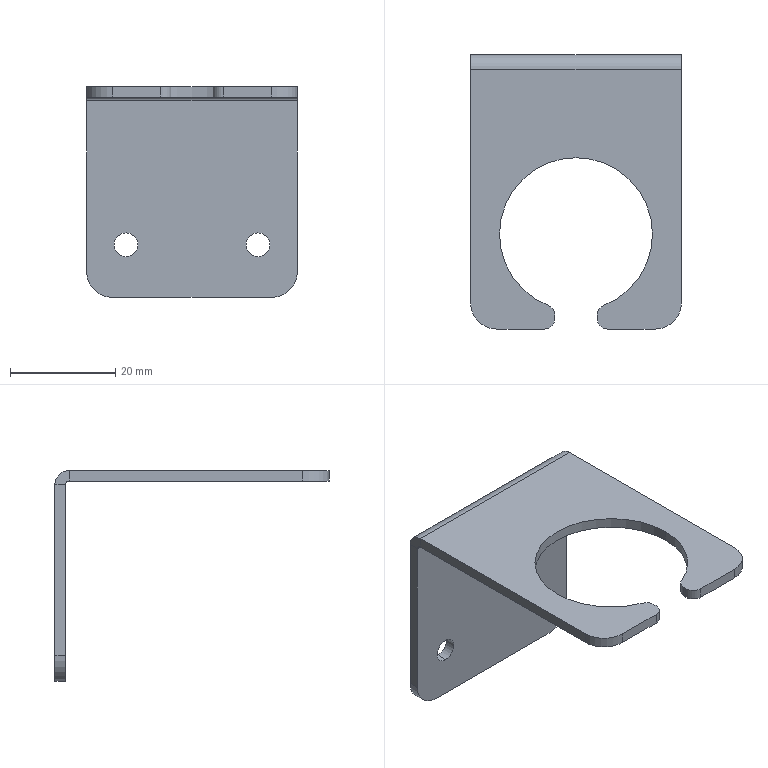Part | STEP file | 02-10 corrugated tube mounting plate (Default) | 1 solid | 32 faces | box 40 x 52 x 40 mm | volume 5649 mm3 | cylinder 17 | plane 15 | commonest cylinder face diameters 4 x4 4.5 x4 10 x4 29 x3 1.473 x1 5.473 x1
STEP:
#1=CARTESIAN_POINT('',(12.5,27.,-32.25));
#2=VERTEX_POINT('',#1);
#3=CARTESIAN_POINT('',(12.5,27.,-27.75));
#4=VERTEX_POINT('',#3);
#5=CARTESIAN_POINT('',(12.5,27.,-30.));
#6=DIRECTION('',(0.,1.,0.));
#7=DIRECTION('',(0.,0.,1.));
#8=AXIS2_PLACEMENT_3D('',#5,#6,#7);
#9=CIRCLE('',#8,2.25);
#10=EDGE_CURVE('',#2,#4,#9,.T.);
#11=ORIENTED_EDGE('',*,*,#10,.T.);
#12=CARTESIAN_POINT('',(12.5,25.,-27.75));
#13=VERTEX_POINT('',#12);
#14=CARTESIAN_POINT('',(12.5,35.,-27.75));
#15=DIRECTION('',(0.,-1.,0.));
#16=VECTOR('',#15,1000.);
#17=LINE('',#14,#16);
#18=EDGE_CURVE('',#4,#13,#17,.T.);
#19=ORIENTED_EDGE('',*,*,#18,.T.);
#20=CARTESIAN_POINT('',(12.5,25.,-32.25));
#21=VERTEX_POINT('',#20);
#22=CARTESIAN_POINT('',(12.5,25.,-30.));
#23=DIRECTION('',(0.,-1.,0.));
#24=DIRECTION('',(0.,0.,1.));
#25=AXIS2_PLACEMENT_3D('',#22,#23,#24);
#26=CIRCLE('',#25,2.25);
#27=EDGE_CURVE('',#13,#21,#26,.T.);
#28=ORIENTED_EDGE('',*,*,#27,.T.);
#29=CARTESIAN_POINT('',(12.5,35.,-32.25));
#30=DIRECTION('',(0.,-1.,0.));
#31=VECTOR('',#30,1000.);
#32=LINE('',#29,#31);
#33=EDGE_CURVE('',#2,#21,#32,.T.);
#34=ORIENTED_EDGE('',*,*,#33,.F.);
#35=EDGE_LOOP('',(#11,#19,#28,#34));
#36=FACE_OUTER_BOUND('',#35,.T.);
#37=CARTESIAN_POINT('',(12.5,35.,-30.));
#38=DIRECTION('',(0.,-1.,0.));
#39=DIRECTION('',(0.,0.,-1.));
#40=AXIS2_PLACEMENT_3D('',#37,#38,#39);
#41=CYLINDRICAL_SURFACE('',#40,2.25);
#42=ADVANCED_FACE('',(#36),#41,.F.);
#43=CARTESIAN_POINT('',(-12.5,27.,-32.25));
#44=VERTEX_POINT('',#43);
#45=CARTESIAN_POINT('',(-12.5,27.,-27.75));
#46=VERTEX_POINT('',#45);
#47=CARTESIAN_POINT('',(-12.5,27.,-30.));
#48=DIRECTION('',(0.,1.,0.));
#49=DIRECTION('',(0.,0.,1.));
#50=AXIS2_PLACEMENT_3D('',#47,#48,#49);
#51=CIRCLE('',#50,2.25);
#52=EDGE_CURVE('',#44,#46,#51,.T.);
#53=ORIENTED_EDGE('',*,*,#52,.T.);
#54=CARTESIAN_POINT('',(-12.5,25.,-27.75));
#55=VERTEX_POINT('',#54);
#56=CARTESIAN_POINT('',(-12.5,35.,-27.75));
#57=DIRECTION('',(0.,-1.,0.));
#58=VECTOR('',#57,1000.);
#59=LINE('',#56,#58);
#60=EDGE_CURVE('',#46,#55,#59,.T.);
#61=ORIENTED_EDGE('',*,*,#60,.T.);
#62=CARTESIAN_POINT('',(-12.5,25.,-32.25));
#63=VERTEX_POINT('',#62);
#64=CARTESIAN_POINT('',(-12.5,25.,-30.));
#65=DIRECTION('',(0.,-1.,0.));
#66=DIRECTION('',(0.,0.,-1.));
#67=AXIS2_PLACEMENT_3D('',#64,#65,#66);
#68=CIRCLE('',#67,2.25);
#69=EDGE_CURVE('',#55,#63,#68,.T.);
#70=ORIENTED_EDGE('',*,*,#69,.T.);
#71=CARTESIAN_POINT('',(-12.5,35.,-32.25));
#72=DIRECTION('',(0.,-1.,0.));
#73=VECTOR('',#72,1000.);
#74=LINE('',#71,#73);
#75=EDGE_CURVE('',#44,#63,#74,.T.);
#76=ORIENTED_EDGE('',*,*,#75,.F.);
#77=EDGE_LOOP('',(#53,#61,#70,#76));
#78=FACE_OUTER_BOUND('',#77,.T.);
#79=CARTESIAN_POINT('',(-12.5,35.,-30.));
#80=DIRECTION('',(0.,-1.,0.));
#81=DIRECTION('',(0.,0.,-1.));
#82=AXIS2_PLACEMENT_3D('',#79,#80,#81);
#83=CYLINDRICAL_SURFACE('',#82,2.25);
#84=ADVANCED_FACE('',(#78),#83,.F.);
#85=CARTESIAN_POINT('',(-14.5,-7.,-2.));
#86=VERTEX_POINT('',#85);
#87=CARTESIAN_POINT('',(-5.273,-20.507,-2.));
#88=VERTEX_POINT('',#87);
#89=CARTESIAN_POINT('',(0.,-7.,-2.));
#90=DIRECTION('',(0.,0.,1.));
#91=DIRECTION('',(1.,0.,0.));
#92=AXIS2_PLACEMENT_3D('',#89,#90,#91);
#93=CIRCLE('',#92,14.5);
#94=EDGE_CURVE('',#86,#88,#93,.T.);
#95=ORIENTED_EDGE('',*,*,#94,.F.);
#96=CARTESIAN_POINT('',(-14.5,-7.,0.));
#97=VERTEX_POINT('',#96);
#98=CARTESIAN_POINT('',(-14.5,-7.,-10.));
#99=DIRECTION('',(0.,0.,1.));
#100=VECTOR('',#99,1000.);
#101=LINE('',#98,#100);
#102=EDGE_CURVE('',#86,#97,#101,.T.);
#103=ORIENTED_EDGE('',*,*,#102,.T.);
#104=CARTESIAN_POINT('',(-5.273,-20.507,0.));
#105=VERTEX_POINT('',#104);
#106=CARTESIAN_POINT('',(0.,-7.,0.));
#107=DIRECTION('',(0.,0.,1.));
#108=DIRECTION('',(1.,0.,0.));
#109=AXIS2_PLACEMENT_3D('',#106,#107,#108);
#110=CIRCLE('',#109,14.5);
#111=EDGE_CURVE('',#97,#105,#110,.T.);
#112=ORIENTED_EDGE('',*,*,#111,.T.);
#113=CARTESIAN_POINT('',(-5.273,-20.507,-10.));
#114=DIRECTION('',(0.,0.,-1.));
#115=VECTOR('',#114,1000.);
#116=LINE('',#113,#115);
#117=EDGE_CURVE('',#105,#88,#116,.T.);
#118=ORIENTED_EDGE('',*,*,#117,.T.);
#119=EDGE_LOOP('',(#95,#103,#112,#118));
#120=FACE_OUTER_BOUND('',#119,.T.);
#121=CARTESIAN_POINT('',(0.,-7.,-10.));
#122=DIRECTION('',(0.,0.,1.));
#123=DIRECTION('',(1.,0.,0.));
#124=AXIS2_PLACEMENT_3D('',#121,#122,#123);
#125=CYLINDRICAL_SURFACE('',#124,14.5);
#126=ADVANCED_FACE('',(#120),#125,.F.);
#127=ORIENTED_EDGE('',*,*,#102,.F.);
#128=CARTESIAN_POINT('',(14.5,-7.,-2.));
#129=VERTEX_POINT('',#128);
#130=CARTESIAN_POINT('',(0.,-7.,-2.));
#131=DIRECTION('',(0.,0.,1.));
#132=DIRECTION('',(1.,0.,0.));
#133=AXIS2_PLACEMENT_3D('',#130,#131,#132);
#134=CIRCLE('',#133,14.5);
#135=EDGE_CURVE('',#129,#86,#134,.T.);
#136=ORIENTED_EDGE('',*,*,#135,.F.);
#137=CARTESIAN_POINT('',(14.5,-7.,0.));
#138=VERTEX_POINT('',#137);
#139=CARTESIAN_POINT('',(14.5,-7.,-10.));
#140=DIRECTION('',(0.,0.,1.));
#141=VECTOR('',#140,1000.);
#142=LINE('',#139,#141);
#143=EDGE_CURVE('',#129,#138,#142,.T.);
#144=ORIENTED_EDGE('',*,*,#143,.T.);
#145=CARTESIAN_POINT('',(0.,-7.,0.));
#146=DIRECTION('',(0.,0.,1.));
#147=DIRECTION('',(1.,0.,0.));
#148=AXIS2_PLACEMENT_3D('',#145,#146,#147);
#149=CIRCLE('',#148,14.5);
#150=EDGE_CURVE('',#138,#97,#149,.T.);
#151=ORIENTED_EDGE('',*,*,#150,.T.);
#152=EDGE_LOOP('',(#127,#136,#144,#151));
#153=FACE_OUTER_BOUND('',#152,.T.);
#154=CARTESIAN_POINT('',(0.,-7.,-10.));
#155=DIRECTION('',(0.,0.,1.));
#156=DIRECTION('',(1.,0.,0.));
#157=AXIS2_PLACEMENT_3D('',#154,#155,#156);
#158=CYLINDRICAL_SURFACE('',#157,14.5);
#159=ADVANCED_FACE('',(#153),#158,.F.);
#160=CARTESIAN_POINT('',(6.,-25.,0.));
#161=VERTEX_POINT('',#160);
#162=CARTESIAN_POINT('',(15.,-25.,0.));
#163=VERTEX_POINT('',#162);
#164=CARTESIAN_POINT('',(-20.,-25.,0.));
#165=DIRECTION('',(1.,0.,0.));
#166=VECTOR('',#165,1000.);
#167=LINE('',#164,#166);
#168=EDGE_CURVE('',#161,#163,#167,.T.);
#169=ORIENTED_EDGE('',*,*,#168,.F.);
#170=CARTESIAN_POINT('',(6.,-25.,-2.));
#171=VERTEX_POINT('',#170);
#172=CARTESIAN_POINT('',(6.,-25.,-2.));
#173=DIRECTION('',(0.,0.,-1.));
#174=VECTOR('',#173,1000.);
#175=LINE('',#172,#174);
#176=EDGE_CURVE('',#161,#171,#175,.T.);
#177=ORIENTED_EDGE('',*,*,#176,.T.);
#178=CARTESIAN_POINT('',(15.,-25.,-2.));
#179=VERTEX_POINT('',#178);
#180=CARTESIAN_POINT('',(-20.,-25.,-2.));
#181=DIRECTION('',(1.,0.,0.));
#182=VECTOR('',#181,1000.);
#183=LINE('',#180,#182);
#184=EDGE_CURVE('',#171,#179,#183,.T.);
#185=ORIENTED_EDGE('',*,*,#184,.T.);
#186=CARTESIAN_POINT('',(15.,-25.,-2.));
#187=DIRECTION('',(0.,0.,1.));
#188=VECTOR('',#187,1000.);
#189=LINE('',#186,#188);
#190=EDGE_CURVE('',#179,#163,#189,.T.);
#191=ORIENTED_EDGE('',*,*,#190,.T.);
#192=EDGE_LOOP('',(#169,#177,#185,#191));
#193=FACE_OUTER_BOUND('',#192,.T.);
#194=CARTESIAN_POINT('',(-20.,-25.,-2.));
#195=DIRECTION('',(0.,-1.,0.));
#196=DIRECTION('',(0.,0.,-1.));
#197=AXIS2_PLACEMENT_3D('',#194,#195,#196);
#198=PLANE('',#197);
#199=ADVANCED_FACE('',(#193),#198,.T.);
#200=CARTESIAN_POINT('',(20.,-20.,0.));
#201=VERTEX_POINT('',#200);
#202=CARTESIAN_POINT('',(20.,24.263,0.));
#203=VERTEX_POINT('',#202);
#204=CARTESIAN_POINT('',(20.,25.,0.));
#205=DIRECTION('',(0.,1.,0.));
#206=VECTOR('',#205,1000.);
#207=LINE('',#204,#206);
#208=EDGE_CURVE('',#201,#203,#207,.T.);
#209=ORIENTED_EDGE('',*,*,#208,.F.);
#210=CARTESIAN_POINT('',(20.,-20.,-2.));
#211=VERTEX_POINT('',#210);
#212=CARTESIAN_POINT('',(20.,-20.,-2.));
#213=DIRECTION('',(0.,0.,-1.));
#214=VECTOR('',#213,1000.);
#215=LINE('',#212,#214);
#216=EDGE_CURVE('',#201,#211,#215,.T.);
#217=ORIENTED_EDGE('',*,*,#216,.T.);
#218=CARTESIAN_POINT('',(20.,24.263,-2.));
#219=VERTEX_POINT('',#218);
#220=CARTESIAN_POINT('',(20.,25.,-2.));
#221=DIRECTION('',(0.,1.,0.));
#222=VECTOR('',#221,1000.);
#223=LINE('',#220,#222);
#224=EDGE_CURVE('',#211,#219,#223,.T.);
#225=ORIENTED_EDGE('',*,*,#224,.T.);
#226=CARTESIAN_POINT('',(20.,24.263,-2.));
#227=DIRECTION('',(0.,0.,1.));
#228=VECTOR('',#227,1000.);
#229=LINE('',#226,#228);
#230=EDGE_CURVE('',#219,#203,#229,.T.);
#231=ORIENTED_EDGE('',*,*,#230,.T.);
#232=EDGE_LOOP('',(#209,#217,#225,#231));
#233=FACE_OUTER_BOUND('',#232,.T.);
#234=CARTESIAN_POINT('',(20.,25.,-2.));
#235=DIRECTION('',(1.,0.,0.));
#236=DIRECTION('',(0.,1.,0.));
#237=AXIS2_PLACEMENT_3D('',#234,#235,#236);
#238=PLANE('',#237);
#239=ADVANCED_FACE('',(#233),#238,.T.);
#240=ORIENTED_EDGE('',*,*,#184,.F.);
#241=CARTESIAN_POINT('',(4.,-23.,-2.));
#242=VERTEX_POINT('',#241);
#243=CARTESIAN_POINT('',(6.,-23.,-2.));
#244=DIRECTION('',(0.,0.,-1.));
#245=DIRECTION('',(1.,0.,0.));
#246=AXIS2_PLACEMENT_3D('',#243,#244,#245);
#247=CIRCLE('',#246,2.);
#248=EDGE_CURVE('',#171,#242,#247,.T.);
#249=ORIENTED_EDGE('',*,*,#248,.T.);
#250=CARTESIAN_POINT('',(4.,-22.37,-2.));
#251=VERTEX_POINT('',#250);
#252=CARTESIAN_POINT('',(4.,-25.,-2.));
#253=DIRECTION('',(0.,1.,0.));
#254=VECTOR('',#253,1000.);
#255=LINE('',#252,#254);
#256=EDGE_CURVE('',#242,#251,#255,.T.);
#257=ORIENTED_EDGE('',*,*,#256,.T.);
#258=CARTESIAN_POINT('',(5.273,-20.507,-2.));
#259=VERTEX_POINT('',#258);
#260=CARTESIAN_POINT('',(6.,-22.37,-2.));
#261=DIRECTION('',(0.,0.,-1.));
#262=DIRECTION('',(1.,0.,0.));
#263=AXIS2_PLACEMENT_3D('',#260,#261,#262);
#264=CIRCLE('',#263,2.);
#265=EDGE_CURVE('',#251,#259,#264,.T.);
#266=ORIENTED_EDGE('',*,*,#265,.T.);
#267=CARTESIAN_POINT('',(0.,-7.,-2.));
#268=DIRECTION('',(0.,0.,1.));
#269=DIRECTION('',(1.,0.,0.));
#270=AXIS2_PLACEMENT_3D('',#267,#268,#269);
#271=CIRCLE('',#270,14.5);
#272=EDGE_CURVE('',#259,#129,#271,.T.);
#273=ORIENTED_EDGE('',*,*,#272,.T.);
#274=ORIENTED_EDGE('',*,*,#135,.T.);
#275=ORIENTED_EDGE('',*,*,#94,.T.);
#276=CARTESIAN_POINT('',(-4.,-22.37,-2.));
#277=VERTEX_POINT('',#276);
#278=CARTESIAN_POINT('',(-6.,-22.37,-2.));
#279=DIRECTION('',(0.,0.,-1.));
#280=DIRECTION('',(1.,0.,0.));
#281=AXIS2_PLACEMENT_3D('',#278,#279,#280);
#282=CIRCLE('',#281,2.);
#283=EDGE_CURVE('',#88,#277,#282,.T.);
#284=ORIENTED_EDGE('',*,*,#283,.T.);
#285=CARTESIAN_POINT('',(-4.,-23.,-2.));
#286=VERTEX_POINT('',#285);
#287=CARTESIAN_POINT('',(-4.,-25.,-2.));
#288=DIRECTION('',(0.,-1.,0.));
#289=VECTOR('',#288,1000.);
#290=LINE('',#287,#289);
#291=EDGE_CURVE('',#277,#286,#290,.T.);
#292=ORIENTED_EDGE('',*,*,#291,.T.);
#293=CARTESIAN_POINT('',(-6.,-25.,-2.));
#294=VERTEX_POINT('',#293);
#295=CARTESIAN_POINT('',(-6.,-23.,-2.));
#296=DIRECTION('',(0.,0.,-1.));
#297=DIRECTION('',(1.,0.,0.));
#298=AXIS2_PLACEMENT_3D('',#295,#296,#297);
#299=CIRCLE('',#298,2.);
#300=EDGE_CURVE('',#286,#294,#299,.T.);
#301=ORIENTED_EDGE('',*,*,#300,.T.);
#302=CARTESIAN_POINT('',(-15.,-25.,-2.));
#303=VERTEX_POINT('',#302);
#304=CARTESIAN_POINT('',(-20.,-25.,-2.));
#305=DIRECTION('',(1.,0.,0.));
#306=VECTOR('',#305,1000.);
#307=LINE('',#304,#306);
#308=EDGE_CURVE('',#303,#294,#307,.T.);
#309=ORIENTED_EDGE('',*,*,#308,.F.);
#310=CARTESIAN_POINT('',(-20.,-20.,-2.));
#311=VERTEX_POINT('',#310);
#312=CARTESIAN_POINT('',(-15.,-20.,-2.));
#313=DIRECTION('',(0.,0.,-1.));
#314=DIRECTION('',(1.,0.,0.));
#315=AXIS2_PLACEMENT_3D('',#312,#313,#314);
#316=CIRCLE('',#315,5.);
#317=EDGE_CURVE('',#303,#311,#316,.T.);
#318=ORIENTED_EDGE('',*,*,#317,.T.);
#319=CARTESIAN_POINT('',(-20.,24.263,-2.));
#320=VERTEX_POINT('',#319);
#321=CARTESIAN_POINT('',(-20.,25.,-2.));
#322=DIRECTION('',(0.,-1.,0.));
#323=VECTOR('',#322,1000.);
#324=LINE('',#321,#323);
#325=EDGE_CURVE('',#320,#311,#324,.T.);
#326=ORIENTED_EDGE('',*,*,#325,.F.);
#327=CARTESIAN_POINT('',(20.,24.263,-2.));
#328=DIRECTION('',(-1.,0.,0.));
#329=VECTOR('',#328,1000.);
#330=LINE('',#327,#329);
#331=EDGE_CURVE('',#219,#320,#330,.T.);
#332=ORIENTED_EDGE('',*,*,#331,.F.);
#333=ORIENTED_EDGE('',*,*,#224,.F.);
#334=CARTESIAN_POINT('',(15.,-20.,-2.));
#335=DIRECTION('',(0.,0.,-1.));
#336=DIRECTION('',(1.,0.,0.));
#337=AXIS2_PLACEMENT_3D('',#334,#335,#336);
#338=CIRCLE('',#337,5.);
#339=EDGE_CURVE('',#211,#179,#338,.T.);
#340=ORIENTED_EDGE('',*,*,#339,.T.);
#341=EDGE_LOOP('',(#240,#249,#257,#266,#273,#274,#275,#284,#292,#301,#309,#318,#326,#332,#333,#340));
#342=FACE_OUTER_BOUND('',#341,.T.);
#343=CARTESIAN_POINT('',(20.,-25.,-2.));
#344=DIRECTION('',(0.,0.,1.));
#345=DIRECTION('',(1.,0.,0.));
#346=AXIS2_PLACEMENT_3D('',#343,#344,#345);
#347=PLANE('',#346);
#348=ADVANCED_FACE('',(#342),#347,.F.);
#349=CARTESIAN_POINT('',(4.,-23.,0.));
#350=VERTEX_POINT('',#349);
#351=CARTESIAN_POINT('',(4.,-22.37,0.));
#352=VERTEX_POINT('',#351);
#353=CARTESIAN_POINT('',(4.,-20.937,0.));
#354=DIRECTION('',(0.,1.,0.));
#355=VECTOR('',#354,1000.);
#356=LINE('',#353,#355);
#357=EDGE_CURVE('',#350,#352,#356,.T.);
#358=ORIENTED_EDGE('',*,*,#357,.F.);
#359=CARTESIAN_POINT('',(6.,-23.,0.));
#360=DIRECTION('',(0.,0.,1.));
#361=DIRECTION('',(1.,0.,0.));
#362=AXIS2_PLACEMENT_3D('',#359,#360,#361);
#363=CIRCLE('',#362,2.);
#364=EDGE_CURVE('',#350,#161,#363,.T.);
#365=ORIENTED_EDGE('',*,*,#364,.T.);
#366=ORIENTED_EDGE('',*,*,#168,.T.);
#367=CARTESIAN_POINT('',(15.,-20.,0.));
#368=DIRECTION('',(0.,0.,1.));
#369=DIRECTION('',(1.,0.,0.));
#370=AXIS2_PLACEMENT_3D('',#367,#368,#369);
#371=CIRCLE('',#370,5.);
#372=EDGE_CURVE('',#163,#201,#371,.T.);
#373=ORIENTED_EDGE('',*,*,#372,.T.);
#374=ORIENTED_EDGE('',*,*,#208,.T.);
#375=CARTESIAN_POINT('',(-20.,24.263,0.));
#376=VERTEX_POINT('',#375);
#377=CARTESIAN_POINT('',(20.,24.263,0.));
#378=DIRECTION('',(-1.,0.,0.));
#379=VECTOR('',#378,1000.);
#380=LINE('',#377,#379);
#381=EDGE_CURVE('',#203,#376,#380,.T.);
#382=ORIENTED_EDGE('',*,*,#381,.T.);
#383=CARTESIAN_POINT('',(-20.,-20.,0.));
#384=VERTEX_POINT('',#383);
#385=CARTESIAN_POINT('',(-20.,25.,0.));
#386=DIRECTION('',(0.,-1.,0.));
#387=VECTOR('',#386,1000.);
#388=LINE('',#385,#387);
#389=EDGE_CURVE('',#376,#384,#388,.T.);
#390=ORIENTED_EDGE('',*,*,#389,.T.);
#391=CARTESIAN_POINT('',(-15.,-25.,0.));
#392=VERTEX_POINT('',#391);
#393=CARTESIAN_POINT('',(-15.,-20.,0.));
#394=DIRECTION('',(0.,0.,1.));
#395=DIRECTION('',(1.,0.,0.));
#396=AXIS2_PLACEMENT_3D('',#393,#394,#395);
#397=CIRCLE('',#396,5.);
#398=EDGE_CURVE('',#384,#392,#397,.T.);
#399=ORIENTED_EDGE('',*,*,#398,.T.);
#400=CARTESIAN_POINT('',(-6.,-25.,0.));
#401=VERTEX_POINT('',#400);
#402=CARTESIAN_POINT('',(-20.,-25.,0.));
#403=DIRECTION('',(1.,0.,0.));
#404=VECTOR('',#403,1000.);
#405=LINE('',#402,#404);
#406=EDGE_CURVE('',#392,#401,#405,.T.);
#407=ORIENTED_EDGE('',*,*,#406,.T.);
#408=CARTESIAN_POINT('',(-4.,-23.,0.));
#409=VERTEX_POINT('',#408);
#410=CARTESIAN_POINT('',(-6.,-23.,0.));
#411=DIRECTION('',(0.,0.,1.));
#412=DIRECTION('',(1.,0.,0.));
#413=AXIS2_PLACEMENT_3D('',#410,#411,#412);
#414=CIRCLE('',#413,2.);
#415=EDGE_CURVE('',#401,#409,#414,.T.);
#416=ORIENTED_EDGE('',*,*,#415,.T.);
#417=CARTESIAN_POINT('',(-4.,-22.37,0.));
#418=VERTEX_POINT('',#417);
#419=CARTESIAN_POINT('',(-4.,-20.937,0.));
#420=DIRECTION('',(0.,-1.,0.));
#421=VECTOR('',#420,1000.);
#422=LINE('',#419,#421);
#423=EDGE_CURVE('',#418,#409,#422,.T.);
#424=ORIENTED_EDGE('',*,*,#423,.F.);
#425=CARTESIAN_POINT('',(-6.,-22.37,0.));
#426=DIRECTION('',(0.,0.,1.));
#427=DIRECTION('',(1.,0.,0.));
#428=AXIS2_PLACEMENT_3D('',#425,#426,#427);
#429=CIRCLE('',#428,2.);
#430=EDGE_CURVE('',#418,#105,#429,.T.);
#431=ORIENTED_EDGE('',*,*,#430,.T.);
#432=ORIENTED_EDGE('',*,*,#111,.F.);
#433=ORIENTED_EDGE('',*,*,#150,.F.);
#434=CARTESIAN_POINT('',(5.273,-20.507,0.));
#435=VERTEX_POINT('',#434);
#436=CARTESIAN_POINT('',(0.,-7.,0.));
#437=DIRECTION('',(0.,0.,1.));
#438=DIRECTION('',(1.,0.,0.));
#439=AXIS2_PLACEMENT_3D('',#436,#437,#438);
#440=CIRCLE('',#439,14.5);
#441=EDGE_CURVE('',#435,#138,#440,.T.);
#442=ORIENTED_EDGE('',*,*,#441,.F.);
#443=CARTESIAN_POINT('',(6.,-22.37,0.));
#444=DIRECTION('',(0.,0.,1.));
#445=DIRECTION('',(1.,0.,0.));
#446=AXIS2_PLACEMENT_3D('',#443,#444,#445);
#447=CIRCLE('',#446,2.);
#448=EDGE_CURVE('',#435,#352,#447,.T.);
#449=ORIENTED_EDGE('',*,*,#448,.T.);
#450=EDGE_LOOP('',(#358,#365,#366,#373,#374,#382,#390,#399,#407,#416,#424,#431,#432,#433,#442,#449));
#451=FACE_OUTER_BOUND('',#450,.T.);
#452=CARTESIAN_POINT('',(20.,-25.,0.));
#453=DIRECTION('',(0.,0.,1.));
#454=DIRECTION('',(1.,0.,0.));
#455=AXIS2_PLACEMENT_3D('',#452,#453,#454);
#456=PLANE('',#455);
#457=ADVANCED_FACE('',(#451),#456,.T.);
#458=ORIENTED_EDGE('',*,*,#308,.T.);
#459=CARTESIAN_POINT('',(-6.,-25.,0.));
#460=DIRECTION('',(0.,0.,1.));
#461=VECTOR('',#460,1000.);
#462=LINE('',#459,#461);
#463=EDGE_CURVE('',#294,#401,#462,.T.);
#464=ORIENTED_EDGE('',*,*,#463,.T.);
#465=ORIENTED_EDGE('',*,*,#406,.F.);
#466=CARTESIAN_POINT('',(-15.,-25.,-2.));
#467=DIRECTION('',(0.,0.,-1.));
#468=VECTOR('',#467,1000.);
#469=LINE('',#466,#468);
#470=EDGE_CURVE('',#392,#303,#469,.T.);
#471=ORIENTED_EDGE('',*,*,#470,.T.);
#472=EDGE_LOOP('',(#458,#464,#465,#471));
#473=FACE_OUTER_BOUND('',#472,.T.);
#474=CARTESIAN_POINT('',(-20.,-25.,-2.));
#475=DIRECTION('',(0.,-1.,0.));
#476=DIRECTION('',(0.,0.,-1.));
#477=AXIS2_PLACEMENT_3D('',#474,#475,#476);
#478=PLANE('',#477);
#479=ADVANCED_FACE('',(#473),#478,.T.);
#480=ORIENTED_EDGE('',*,*,#325,.T.);
#481=CARTESIAN_POINT('',(-20.,-20.,-2.));
#482=DIRECTION('',(0.,0.,1.));
#483=VECTOR('',#482,1000.);
#484=LINE('',#481,#483);
#485=EDGE_CURVE('',#311,#384,#484,.T.);
#486=ORIENTED_EDGE('',*,*,#485,.T.);
#487=ORIENTED_EDGE('',*,*,#389,.F.);
#488=CARTESIAN_POINT('',(-20.,24.263,-2.));
#489=DIRECTION('',(0.,0.,1.));
#490=VECTOR('',#489,1000.);
#491=LINE('',#488,#490);
#492=EDGE_CURVE('',#320,#376,#491,.T.);
#493=ORIENTED_EDGE('',*,*,#492,.F.);
#494=EDGE_LOOP('',(#480,#486,#487,#493));
#495=FACE_OUTER_BOUND('',#494,.T.);
#496=CARTESIAN_POINT('',(-20.,25.,-2.));
#497=DIRECTION('',(-1.,0.,0.));
#498=DIRECTION('',(0.,-1.,0.));
#499=AXIS2_PLACEMENT_3D('',#496,#497,#498);
#500=PLANE('',#499);
#501=ADVANCED_FACE('',(#495),#500,.T.);
#502=CARTESIAN_POINT('',(-20.,25.,-2.737));
#503=VERTEX_POINT('',#502);
#504=CARTESIAN_POINT('',(-20.,27.,-2.737));
#505=VERTEX_POINT('',#504);
#506=CARTESIAN_POINT('',(-20.,25.,-2.737));
#507=DIRECTION('',(0.,1.,0.));
#508=VECTOR('',#507,1000.);
#509=LINE('',#506,#508);
#510=EDGE_CURVE('',#503,#505,#509,.T.);
#511=ORIENTED_EDGE('',*,*,#510,.F.);
#512=CARTESIAN_POINT('',(-20.,24.263,-2.737));
#513=DIRECTION('',(-1.,0.,0.));
#514=DIRECTION('',(0.,0.,-1.));
#515=AXIS2_PLACEMENT_3D('',#512,#513,#514);
#516=CIRCLE('',#515,0.7366);
#517=EDGE_CURVE('',#320,#503,#516,.T.);
#518=ORIENTED_EDGE('',*,*,#517,.F.);
#519=ORIENTED_EDGE('',*,*,#492,.T.);
#520=CARTESIAN_POINT('',(-20.,24.263,-2.737));
#521=DIRECTION('',(-1.,0.,0.));
#522=DIRECTION('',(0.,0.,-1.));
#523=AXIS2_PLACEMENT_3D('',#520,#521,#522);
#524=CIRCLE('',#523,2.737);
#525=EDGE_CURVE('',#376,#505,#524,.T.);
#526=ORIENTED_EDGE('',*,*,#525,.T.);
#527=EDGE_LOOP('',(#511,#518,#519,#526));
#528=FACE_OUTER_BOUND('',#527,.T.);
#529=CARTESIAN_POINT('',(-20.,24.263,-2.737));
#530=DIRECTION('',(-1.,0.,0.));
#531=DIRECTION('',(0.,0.,1.));
#532=AXIS2_PLACEMENT_3D('',#529,#530,#531);
#533=PLANE('',#532);
#534=ADVANCED_FACE('',(#528),#533,.T.);
#535=CARTESIAN_POINT('',(20.,25.,-2.737));
#536=VERTEX_POINT('',#535);
#537=CARTESIAN_POINT('',(20.,24.263,-2.737));
#538=DIRECTION('',(1.,0.,0.));
#539=DIRECTION('',(0.,0.,-1.));
#540=AXIS2_PLACEMENT_3D('',#537,#538,#539);
#541=CIRCLE('',#540,0.7366);
#542=EDGE_CURVE('',#536,#219,#541,.T.);
#543=ORIENTED_EDGE('',*,*,#542,.F.);
#544=CARTESIAN_POINT('',(20.,27.,-2.737));
#545=VERTEX_POINT('',#544);
#546=CARTESIAN_POINT('',(20.,25.,-2.737));
#547=DIRECTION('',(0.,1.,0.));
#548=VECTOR('',#547,1000.);
#549=LINE('',#546,#548);
#550=EDGE_CURVE('',#536,#545,#549,.T.);
#551=ORIENTED_EDGE('',*,*,#550,.T.);
#552=CARTESIAN_POINT('',(20.,24.263,-2.737));
#553=DIRECTION('',(1.,0.,0.));
#554=DIRECTION('',(0.,0.,-1.));
#555=AXIS2_PLACEMENT_3D('',#552,#553,#554);
#556=CIRCLE('',#555,2.737);
#557=EDGE_CURVE('',#545,#203,#556,.T.);
#558=ORIENTED_EDGE('',*,*,#557,.T.);
#559=ORIENTED_EDGE('',*,*,#230,.F.);
#560=EDGE_LOOP('',(#543,#551,#558,#559));
#561=FACE_OUTER_BOUND('',#560,.T.);
#562=CARTESIAN_POINT('',(20.,24.263,-2.737));
#563=DIRECTION('',(-1.,0.,0.));
#564=DIRECTION('',(0.,0.,1.));
#565=AXIS2_PLACEMENT_3D('',#562,#563,#564);
#566=PLANE('',#565);
#567=ADVANCED_FACE('',(#561),#566,.F.);
#568=ORIENTED_EDGE('',*,*,#381,.F.);
#569=ORIENTED_EDGE('',*,*,#557,.F.);
#570=CARTESIAN_POINT('',(20.,27.,-2.737));
#571=DIRECTION('',(1.,0.,0.));
#572=VECTOR('',#571,1000.);
#573=LINE('',#570,#572);
#574=EDGE_CURVE('',#505,#545,#573,.T.);
#575=ORIENTED_EDGE('',*,*,#574,.F.);
#576=ORIENTED_EDGE('',*,*,#525,.F.);
#577=EDGE_LOOP('',(#568,#569,#575,#576));
#578=FACE_OUTER_BOUND('',#577,.T.);
#579=CARTESIAN_POINT('',(20.,24.263,-2.737));
#580=DIRECTION('',(1.,0.,0.));
#581=DIRECTION('',(0.,1.,0.));
#582=AXIS2_PLACEMENT_3D('',#579,#580,#581);
#583=CYLINDRICAL_SURFACE('',#582,2.737);
#584=ADVANCED_FACE('',(#578),#583,.T.);
#585=ORIENTED_EDGE('',*,*,#331,.T.);
#586=ORIENTED_EDGE('',*,*,#517,.T.);
#587=CARTESIAN_POINT('',(-20.,25.,-2.737));
#588=DIRECTION('',(1.,0.,0.));
#589=VECTOR('',#588,1000.);
#590=LINE('',#587,#589);
#591=EDGE_CURVE('',#503,#536,#590,.T.);
#592=ORIENTED_EDGE('',*,*,#591,.T.);
#593=ORIENTED_EDGE('',*,*,#542,.T.);
#594=EDGE_LOOP('',(#585,#586,#592,#593));
#595=FACE_OUTER_BOUND('',#594,.T.);
#596=CARTESIAN_POINT('',(20.,24.263,-2.737));
#597=DIRECTION('',(1.,0.,0.));
#598=DIRECTION('',(0.,1.,0.));
#599=AXIS2_PLACEMENT_3D('',#596,#597,#598);
#600=CYLINDRICAL_SURFACE('',#599,0.7366);
#601=ADVANCED_FACE('',(#595),#600,.F.);
#602=CARTESIAN_POINT('',(20.,25.,-35.));
#603=VERTEX_POINT('',#602);
#604=CARTESIAN_POINT('',(20.,25.,-2.));
#605=DIRECTION('',(0.,0.,1.));
#606=VECTOR('',#605,1000.);
#607=LINE('',#604,#606);
#608=EDGE_CURVE('',#603,#536,#607,.T.);
#609=ORIENTED_EDGE('',*,*,#608,.F.);
#610=CARTESIAN_POINT('',(20.,27.,-35.));
#611=VERTEX_POINT('',#610);
#612=CARTESIAN_POINT('',(20.,27.,-35.));
#613=DIRECTION('',(0.,1.,0.));
#614=VECTOR('',#613,1000.);
#615=LINE('',#612,#614);
#616=EDGE_CURVE('',#603,#611,#615,.T.);
#617=ORIENTED_EDGE('',*,*,#616,.T.);
#618=CARTESIAN_POINT('',(20.,27.,-2.));
#619=DIRECTION('',(0.,0.,1.));
#620=VECTOR('',#619,1000.);
#621=LINE('',#618,#620);
#622=EDGE_CURVE('',#611,#545,#621,.T.);
#623=ORIENTED_EDGE('',*,*,#622,.T.);
#624=ORIENTED_EDGE('',*,*,#550,.F.);
#625=EDGE_LOOP('',(#609,#617,#623,#624));
#626=FACE_OUTER_BOUND('',#625,.T.);
#627=CARTESIAN_POINT('',(20.,27.,-2.));
#628=DIRECTION('',(1.,0.,0.));
#629=DIRECTION('',(0.,0.,-1.));
#630=AXIS2_PLACEMENT_3D('',#627,#628,#629);
#631=PLANE('',#630);
#632=ADVANCED_FACE('',(#626),#631,.T.);
#633=CARTESIAN_POINT('',(-20.,27.,-35.));
#634=VERTEX_POINT('',#633);
#635=CARTESIAN_POINT('',(-20.,27.,-40.));
#636=DIRECTION('',(0.,0.,-1.));
#637=VECTOR('',#636,1000.);
#638=LINE('',#635,#637);
#639=EDGE_CURVE('',#505,#634,#638,.T.);
#640=ORIENTED_EDGE('',*,*,#639,.T.);
#641=CARTESIAN_POINT('',(-20.,25.,-35.));
#642=VERTEX_POINT('',#641);
#643=CARTESIAN_POINT('',(-20.,27.,-35.));
#644=DIRECTION('',(0.,-1.,0.));
#645=VECTOR('',#644,1000.);
#646=LINE('',#643,#645);
#647=EDGE_CURVE('',#634,#642,#646,.T.);
#648=ORIENTED_EDGE('',*,*,#647,.T.);
#649=CARTESIAN_POINT('',(-20.,25.,-40.));
#650=DIRECTION('',(0.,0.,-1.));
#651=VECTOR('',#650,1000.);
#652=LINE('',#649,#651);
#653=EDGE_CURVE('',#503,#642,#652,.T.);
#654=ORIENTED_EDGE('',*,*,#653,.F.);
#655=ORIENTED_EDGE('',*,*,#510,.T.);
#656=EDGE_LOOP('',(#640,#648,#654,#655));
#657=FACE_OUTER_BOUND('',#656,.T.);
#658=CARTESIAN_POINT('',(-20.,27.,-40.));
#659=DIRECTION('',(-1.,0.,0.));
#660=DIRECTION('',(0.,0.,1.));
#661=AXIS2_PLACEMENT_3D('',#658,#659,#660);
#662=PLANE('',#661);
#663=ADVANCED_FACE('',(#657),#662,.T.);
#664=ORIENTED_EDGE('',*,*,#10,.F.);
#665=CARTESIAN_POINT('',(12.5,27.,-30.));
#666=DIRECTION('',(0.,1.,0.));
#667=DIRECTION('',(0.,0.,1.));
#668=AXIS2_PLACEMENT_3D('',#665,#666,#667);
#669=CIRCLE('',#668,2.25);
#670=EDGE_CURVE('',#4,#2,#669,.T.);
#671=ORIENTED_EDGE('',*,*,#670,.F.);
#672=EDGE_LOOP('',(#664,#671));
#673=FACE_BOUND('',#672,.T.);
#674=ORIENTED_EDGE('',*,*,#52,.F.);
#675=CARTESIAN_POINT('',(-12.5,27.,-30.));
#676=DIRECTION('',(0.,1.,0.));
#677=DIRECTION('',(0.,0.,1.));
#678=AXIS2_PLACEMENT_3D('',#675,#676,#677);
#679=CIRCLE('',#678,2.25);
#680=EDGE_CURVE('',#46,#44,#679,.T.);
#681=ORIENTED_EDGE('',*,*,#680,.F.);
#682=EDGE_LOOP('',(#674,#681));
#683=FACE_BOUND('',#682,.T.);
#684=CARTESIAN_POINT('',(-15.,27.,-40.));
#685=VERTEX_POINT('',#684);
#686=CARTESIAN_POINT('',(15.,27.,-40.));
#687=VERTEX_POINT('',#686);
#688=CARTESIAN_POINT('',(20.,27.,-40.));
#689=DIRECTION('',(1.,0.,0.));
#690=VECTOR('',#689,1000.);
#691=LINE('',#688,#690);
#692=EDGE_CURVE('',#685,#687,#691,.T.);
#693=ORIENTED_EDGE('',*,*,#692,.F.);
#694=CARTESIAN_POINT('',(-15.,27.,-35.));
#695=DIRECTION('',(0.,1.,0.));
#696=DIRECTION('',(0.,0.,1.));
#697=AXIS2_PLACEMENT_3D('',#694,#695,#696);
#698=CIRCLE('',#697,5.);
#699=EDGE_CURVE('',#685,#634,#698,.T.);
#700=ORIENTED_EDGE('',*,*,#699,.T.);
#701=ORIENTED_EDGE('',*,*,#639,.F.);
#702=ORIENTED_EDGE('',*,*,#574,.T.);
#703=ORIENTED_EDGE('',*,*,#622,.F.);
#704=CARTESIAN_POINT('',(15.,27.,-35.));
#705=DIRECTION('',(0.,1.,0.));
#706=DIRECTION('',(0.,0.,1.));
#707=AXIS2_PLACEMENT_3D('',#704,#705,#706);
#708=CIRCLE('',#707,5.);
#709=EDGE_CURVE('',#611,#687,#708,.T.);
#710=ORIENTED_EDGE('',*,*,#709,.T.);
#711=EDGE_LOOP('',(#693,#700,#701,#702,#703,#710));
#712=FACE_OUTER_BOUND('',#711,.T.);
#713=CARTESIAN_POINT('',(20.,27.,-2.));
#714=DIRECTION('',(0.,1.,0.));
#715=DIRECTION('',(0.,0.,1.));
#716=AXIS2_PLACEMENT_3D('',#713,#714,#715);
#717=PLANE('',#716);
#718=ADVANCED_FACE('',(#673,#683,#712),#717,.T.);
#719=CARTESIAN_POINT('',(12.5,25.,-30.));
#720=DIRECTION('',(0.,-1.,0.));
#721=DIRECTION('',(0.,0.,1.));
#722=AXIS2_PLACEMENT_3D('',#719,#720,#721);
#723=CIRCLE('',#722,2.25);
#724=EDGE_CURVE('',#21,#13,#723,.T.);
#725=ORIENTED_EDGE('',*,*,#724,.F.);
#726=ORIENTED_EDGE('',*,*,#27,.F.);
#727=EDGE_LOOP('',(#725,#726));
#728=FACE_BOUND('',#727,.T.);
#729=CARTESIAN_POINT('',(-12.5,25.,-30.));
#730=DIRECTION('',(0.,-1.,0.));
#731=DIRECTION('',(0.,0.,-1.));
#732=AXIS2_PLACEMENT_3D('',#729,#730,#731);
#733=CIRCLE('',#732,2.25);
#734=EDGE_CURVE('',#63,#55,#733,.T.);
#735=ORIENTED_EDGE('',*,*,#734,.F.);
#736=ORIENTED_EDGE('',*,*,#69,.F.);
#737=EDGE_LOOP('',(#735,#736));
#738=FACE_BOUND('',#737,.T.);
#739=ORIENTED_EDGE('',*,*,#653,.T.);
#740=CARTESIAN_POINT('',(-15.,25.,-40.));
#741=VERTEX_POINT('',#740);
#742=CARTESIAN_POINT('',(-15.,25.,-35.));
#743=DIRECTION('',(0.,-1.,0.));
#744=DIRECTION('',(0.,0.,1.));
#745=AXIS2_PLACEMENT_3D('',#742,#743,#744);
#746=CIRCLE('',#745,5.);
#747=EDGE_CURVE('',#642,#741,#746,.T.);
#748=ORIENTED_EDGE('',*,*,#747,.T.);
#749=CARTESIAN_POINT('',(15.,25.,-40.));
#750=VERTEX_POINT('',#749);
#751=CARTESIAN_POINT('',(20.,25.,-40.));
#752=DIRECTION('',(1.,0.,0.));
#753=VECTOR('',#752,1000.);
#754=LINE('',#751,#753);
#755=EDGE_CURVE('',#741,#750,#754,.T.);
#756=ORIENTED_EDGE('',*,*,#755,.T.);
#757=CARTESIAN_POINT('',(15.,25.,-35.));
#758=DIRECTION('',(0.,-1.,0.));
#759=DIRECTION('',(0.,0.,1.));
#760=AXIS2_PLACEMENT_3D('',#757,#758,#759);
#761=CIRCLE('',#760,5.);
#762=EDGE_CURVE('',#750,#603,#761,.T.);
#763=ORIENTED_EDGE('',*,*,#762,.T.);
#764=ORIENTED_EDGE('',*,*,#608,.T.);
#765=ORIENTED_EDGE('',*,*,#591,.F.);
#766=EDGE_LOOP('',(#739,#748,#756,#763,#764,#765));
#767=FACE_OUTER_BOUND('',#766,.T.);
#768=CARTESIAN_POINT('',(20.,25.,-2.));
#769=DIRECTION('',(0.,1.,0.));
#770=DIRECTION('',(0.,0.,1.));
#771=AXIS2_PLACEMENT_3D('',#768,#769,#770);
#772=PLANE('',#771);
#773=ADVANCED_FACE('',(#728,#738,#767),#772,.F.);
#774=ORIENTED_EDGE('',*,*,#755,.F.);
#775=CARTESIAN_POINT('',(-15.,27.,-40.));
#776=DIRECTION('',(0.,1.,0.));
#777=VECTOR('',#776,1000.);
#778=LINE('',#775,#777);
#779=EDGE_CURVE('',#741,#685,#778,.T.);
#780=ORIENTED_EDGE('',*,*,#779,.T.);
#781=ORIENTED_EDGE('',*,*,#692,.T.);
#782=CARTESIAN_POINT('',(15.,27.,-40.));
#783=DIRECTION('',(0.,-1.,0.));
#784=VECTOR('',#783,1000.);
#785=LINE('',#782,#784);
#786=EDGE_CURVE('',#687,#750,#785,.T.);
#787=ORIENTED_EDGE('',*,*,#786,.T.);
#788=EDGE_LOOP('',(#774,#780,#781,#787));
#789=FACE_OUTER_BOUND('',#788,.T.);
#790=CARTESIAN_POINT('',(20.,27.,-40.));
#791=DIRECTION('',(0.,0.,-1.));
#792=DIRECTION('',(0.,1.,0.));
#793=AXIS2_PLACEMENT_3D('',#790,#791,#792);
#794=PLANE('',#793);
#795=ADVANCED_FACE('',(#789),#794,.T.);
#796=ORIENTED_EDGE('',*,*,#143,.F.);
#797=ORIENTED_EDGE('',*,*,#272,.F.);
#798=CARTESIAN_POINT('',(5.273,-20.507,-10.));
#799=DIRECTION('',(0.,0.,1.));
#800=VECTOR('',#799,1000.);
#801=LINE('',#798,#800);
#802=EDGE_CURVE('',#259,#435,#801,.T.);
#803=ORIENTED_EDGE('',*,*,#802,.T.);
#804=ORIENTED_EDGE('',*,*,#441,.T.);
#805=EDGE_LOOP('',(#796,#797,#803,#804));
#806=FACE_OUTER_BOUND('',#805,.T.);
#807=CARTESIAN_POINT('',(0.,-7.,-10.));
#808=DIRECTION('',(0.,0.,1.));
#809=DIRECTION('',(1.,0.,0.));
#810=AXIS2_PLACEMENT_3D('',#807,#808,#809);
#811=CYLINDRICAL_SURFACE('',#810,14.5);
#812=ADVANCED_FACE('',(#806),#811,.F.);
#813=ORIENTED_EDGE('',*,*,#256,.F.);
#814=CARTESIAN_POINT('',(4.,-23.,0.));
#815=DIRECTION('',(0.,0.,1.));
#816=VECTOR('',#815,1000.);
#817=LINE('',#814,#816);
#818=EDGE_CURVE('',#242,#350,#817,.T.);
#819=ORIENTED_EDGE('',*,*,#818,.T.);
#820=ORIENTED_EDGE('',*,*,#357,.T.);
#821=CARTESIAN_POINT('',(4.,-22.37,-10.));
#822=DIRECTION('',(0.,0.,-1.));
#823=VECTOR('',#822,1000.);
#824=LINE('',#821,#823);
#825=EDGE_CURVE('',#352,#251,#824,.T.);
#826=ORIENTED_EDGE('',*,*,#825,.T.);
#827=EDGE_LOOP('',(#813,#819,#820,#826));
#828=FACE_OUTER_BOUND('',#827,.T.);
#829=CARTESIAN_POINT('',(4.,-20.937,-10.));
#830=DIRECTION('',(1.,0.,0.));
#831=DIRECTION('',(0.,1.,0.));
#832=AXIS2_PLACEMENT_3D('',#829,#830,#831);
#833=PLANE('',#832);
#834=ADVANCED_FACE('',(#828),#833,.F.);
#835=ORIENTED_EDGE('',*,*,#423,.T.);
#836=CARTESIAN_POINT('',(-4.,-23.,-2.));
#837=DIRECTION('',(0.,0.,-1.));
#838=VECTOR('',#837,1000.);
#839=LINE('',#836,#838);
#840=EDGE_CURVE('',#409,#286,#839,.T.);
#841=ORIENTED_EDGE('',*,*,#840,.T.);
#842=ORIENTED_EDGE('',*,*,#291,.F.);
#843=CARTESIAN_POINT('',(-4.,-22.37,-10.));
#844=DIRECTION('',(0.,0.,1.));
#845=VECTOR('',#844,1000.);
#846=LINE('',#843,#845);
#847=EDGE_CURVE('',#277,#418,#846,.T.);
#848=ORIENTED_EDGE('',*,*,#847,.T.);
#849=EDGE_LOOP('',(#835,#841,#842,#848));
#850=FACE_OUTER_BOUND('',#849,.T.);
#851=CARTESIAN_POINT('',(-4.,-20.937,-10.));
#852=DIRECTION('',(-1.,0.,0.));
#853=DIRECTION('',(0.,-1.,0.));
#854=AXIS2_PLACEMENT_3D('',#851,#852,#853);
#855=PLANE('',#854);
#856=ADVANCED_FACE('',(#850),#855,.F.);
#857=ORIENTED_EDGE('',*,*,#699,.F.);
#858=ORIENTED_EDGE('',*,*,#779,.F.);
#859=ORIENTED_EDGE('',*,*,#747,.F.);
#860=ORIENTED_EDGE('',*,*,#647,.F.);
#861=EDGE_LOOP('',(#857,#858,#859,#860));
#862=FACE_OUTER_BOUND('',#861,.T.);
#863=CARTESIAN_POINT('',(-15.,27.,-35.));
#864=DIRECTION('',(0.,-1.,0.));
#865=DIRECTION('',(0.,0.,-1.));
#866=AXIS2_PLACEMENT_3D('',#863,#864,#865);
#867=CYLINDRICAL_SURFACE('',#866,5.);
#868=ADVANCED_FACE('',(#862),#867,.T.);
#869=ORIENTED_EDGE('',*,*,#709,.F.);
#870=ORIENTED_EDGE('',*,*,#616,.F.);
#871=ORIENTED_EDGE('',*,*,#762,.F.);
#872=ORIENTED_EDGE('',*,*,#786,.F.);
#873=EDGE_LOOP('',(#869,#870,#871,#872));
#874=FACE_OUTER_BOUND('',#873,.T.);
#875=CARTESIAN_POINT('',(15.,27.,-35.));
#876=DIRECTION('',(0.,-1.,0.));
#877=DIRECTION('',(0.,0.,-1.));
#878=AXIS2_PLACEMENT_3D('',#875,#876,#877);
#879=CYLINDRICAL_SURFACE('',#878,5.);
#880=ADVANCED_FACE('',(#874),#879,.T.);
#881=ORIENTED_EDGE('',*,*,#339,.F.);
#882=ORIENTED_EDGE('',*,*,#216,.F.);
#883=ORIENTED_EDGE('',*,*,#372,.F.);
#884=ORIENTED_EDGE('',*,*,#190,.F.);
#885=EDGE_LOOP('',(#881,#882,#883,#884));
#886=FACE_OUTER_BOUND('',#885,.T.);
#887=CARTESIAN_POINT('',(15.,-20.,-2.));
#888=DIRECTION('',(0.,0.,1.));
#889=DIRECTION('',(1.,0.,0.));
#890=AXIS2_PLACEMENT_3D('',#887,#888,#889);
#891=CYLINDRICAL_SURFACE('',#890,5.);
#892=ADVANCED_FACE('',(#886),#891,.T.);
#893=ORIENTED_EDGE('',*,*,#317,.F.);
#894=ORIENTED_EDGE('',*,*,#470,.F.);
#895=ORIENTED_EDGE('',*,*,#398,.F.);
#896=ORIENTED_EDGE('',*,*,#485,.F.);
#897=EDGE_LOOP('',(#893,#894,#895,#896));
#898=FACE_OUTER_BOUND('',#897,.T.);
#899=CARTESIAN_POINT('',(-15.,-20.,-2.));
#900=DIRECTION('',(0.,0.,1.));
#901=DIRECTION('',(1.,0.,0.));
#902=AXIS2_PLACEMENT_3D('',#899,#900,#901);
#903=CYLINDRICAL_SURFACE('',#902,5.);
#904=ADVANCED_FACE('',(#898),#903,.T.);
#905=ORIENTED_EDGE('',*,*,#248,.F.);
#906=ORIENTED_EDGE('',*,*,#176,.F.);
#907=ORIENTED_EDGE('',*,*,#364,.F.);
#908=ORIENTED_EDGE('',*,*,#818,.F.);
#909=EDGE_LOOP('',(#905,#906,#907,#908));
#910=FACE_OUTER_BOUND('',#909,.T.);
#911=CARTESIAN_POINT('',(6.,-23.,-10.));
#912=DIRECTION('',(0.,0.,-1.));
#913=DIRECTION('',(-1.,0.,0.));
#914=AXIS2_PLACEMENT_3D('',#911,#912,#913);
#915=CYLINDRICAL_SURFACE('',#914,2.);
#916=ADVANCED_FACE('',(#910),#915,.T.);
#917=ORIENTED_EDGE('',*,*,#415,.F.);
#918=ORIENTED_EDGE('',*,*,#463,.F.);
#919=ORIENTED_EDGE('',*,*,#300,.F.);
#920=ORIENTED_EDGE('',*,*,#840,.F.);
#921=EDGE_LOOP('',(#917,#918,#919,#920));
#922=FACE_OUTER_BOUND('',#921,.T.);
#923=CARTESIAN_POINT('',(-6.,-23.,-10.));
#924=DIRECTION('',(0.,0.,1.));
#925=DIRECTION('',(1.,0.,0.));
#926=AXIS2_PLACEMENT_3D('',#923,#924,#925);
#927=CYLINDRICAL_SURFACE('',#926,2.);
#928=ADVANCED_FACE('',(#922),#927,.T.);
#929=ORIENTED_EDGE('',*,*,#265,.F.);
#930=ORIENTED_EDGE('',*,*,#825,.F.);
#931=ORIENTED_EDGE('',*,*,#448,.F.);
#932=ORIENTED_EDGE('',*,*,#802,.F.);
#933=EDGE_LOOP('',(#929,#930,#931,#932));
#934=FACE_OUTER_BOUND('',#933,.T.);
#935=CARTESIAN_POINT('',(6.,-22.37,-10.));
#936=DIRECTION('',(0.,0.,1.));
#937=DIRECTION('',(1.,0.,0.));
#938=AXIS2_PLACEMENT_3D('',#935,#936,#937);
#939=CYLINDRICAL_SURFACE('',#938,2.);
#940=ADVANCED_FACE('',(#934),#939,.T.);
#941=ORIENTED_EDGE('',*,*,#283,.F.);
#942=ORIENTED_EDGE('',*,*,#117,.F.);
#943=ORIENTED_EDGE('',*,*,#430,.F.);
#944=ORIENTED_EDGE('',*,*,#847,.F.);
#945=EDGE_LOOP('',(#941,#942,#943,#944));
#946=FACE_OUTER_BOUND('',#945,.T.);
#947=CARTESIAN_POINT('',(-6.,-22.37,-10.));
#948=DIRECTION('',(0.,0.,1.));
#949=DIRECTION('',(1.,0.,0.));
#950=AXIS2_PLACEMENT_3D('',#947,#948,#949);
#951=CYLINDRICAL_SURFACE('',#950,2.);
#952=ADVANCED_FACE('',(#946),#951,.T.);
#953=ORIENTED_EDGE('',*,*,#60,.F.);
#954=ORIENTED_EDGE('',*,*,#680,.T.);
#955=ORIENTED_EDGE('',*,*,#75,.T.);
#956=ORIENTED_EDGE('',*,*,#734,.T.);
#957=EDGE_LOOP('',(#953,#954,#955,#956));
#958=FACE_OUTER_BOUND('',#957,.T.);
#959=CARTESIAN_POINT('',(-12.5,35.,-30.));
#960=DIRECTION('',(0.,-1.,0.));
#961=DIRECTION('',(0.,0.,-1.));
#962=AXIS2_PLACEMENT_3D('',#959,#960,#961);
#963=CYLINDRICAL_SURFACE('',#962,2.25);
#964=ADVANCED_FACE('',(#958),#963,.F.);
#965=ORIENTED_EDGE('',*,*,#18,.F.);
#966=ORIENTED_EDGE('',*,*,#670,.T.);
#967=ORIENTED_EDGE('',*,*,#33,.T.);
#968=ORIENTED_EDGE('',*,*,#724,.T.);
#969=EDGE_LOOP('',(#965,#966,#967,#968));
#970=FACE_OUTER_BOUND('',#969,.T.);
#971=CARTESIAN_POINT('',(12.5,35.,-30.));
#972=DIRECTION('',(0.,-1.,0.));
#973=DIRECTION('',(0.,0.,-1.));
#974=AXIS2_PLACEMENT_3D('',#971,#972,#973);
#975=CYLINDRICAL_SURFACE('',#974,2.25);
#976=ADVANCED_FACE('',(#970),#975,.F.);
#977=CLOSED_SHELL('',(#42,#84,#126,#159,#199,#239,#348,#457,#479,#501,#534,#567,#584,#601,#632,#663,#718,#773,#795,#812,#834,#856,#868,#880,#892,#904,#916,#928,#940,#952,#964,#976));
#978=MANIFOLD_SOLID_BREP('',#977);
#979=CARTESIAN_POINT('',(0.,0.,0.));
#980=DIRECTION('',(0.,0.,1.));
#981=DIRECTION('',(1.,0.,0.));
#982=AXIS2_PLACEMENT_3D('',#979,#980,#981);
#983=(LENGTH_UNIT()NAMED_UNIT(*)SI_UNIT(.MILLI.,.METRE.));
#984=UNCERTAINTY_MEASURE_WITH_UNIT(LENGTH_MEASURE(0.00001),#983,'','');
#985=(NAMED_UNIT(*)PLANE_ANGLE_UNIT()SI_UNIT($,.RADIAN.));
#986=(NAMED_UNIT(*)SI_UNIT($,.STERADIAN.)SOLID_ANGLE_UNIT());
#987=(GEOMETRIC_REPRESENTATION_CONTEXT(3)GLOBAL_UNCERTAINTY_ASSIGNED_CONTEXT((#984))GLOBAL_UNIT_ASSIGNED_CONTEXT((#983,#985,#986))REPRESENTATION_CONTEXT('',''));
#988=ADVANCED_BREP_SHAPE_REPRESENTATION('',(#978,#982),#987);